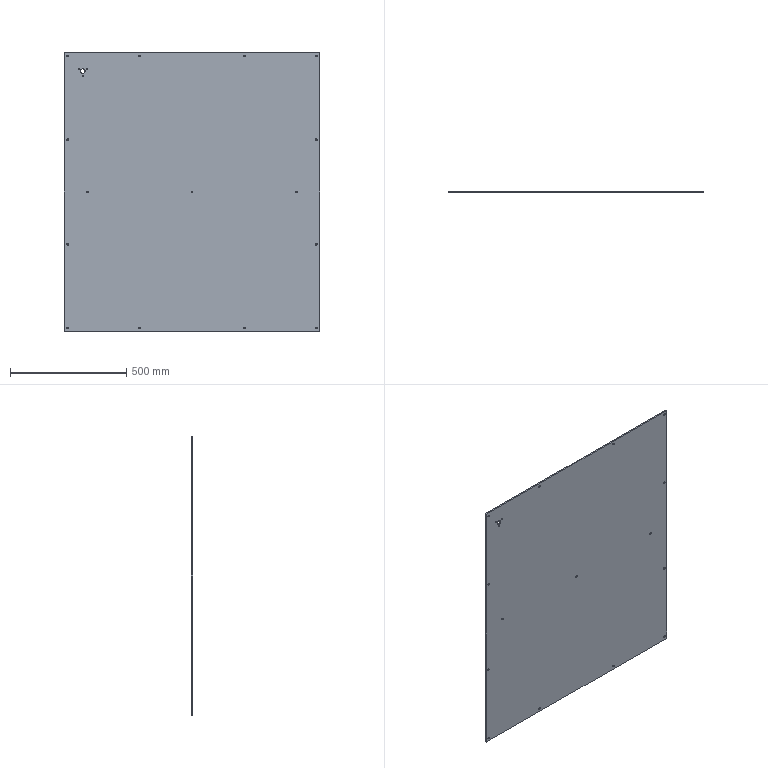Part | SolidWorks | features HoleWzd 2, ICE 2, Extrusion 1, Fillet 1 | 1 solid | 48 faces | box 1100 x 6 x 1200 mm | volume 7913109 mm3 | cylinder 42 | plane 6 | commonest cylinder face diameters 8 x30 5 x6 10 x4 20 x2